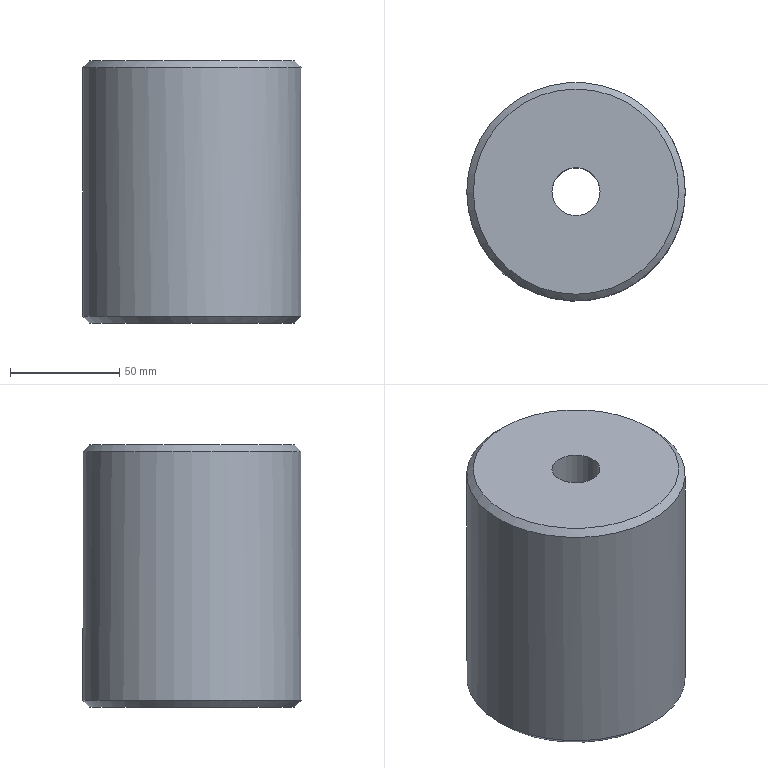Part | STEP file | solid 80 | 1 solid | 8 faces | box 100 x 100 x 120 mm | volume 885185 mm3 | plane 3 | cylinder 3 | cone 2 | commonest cylinder face diameters 22 x1 32 x1 100 x1